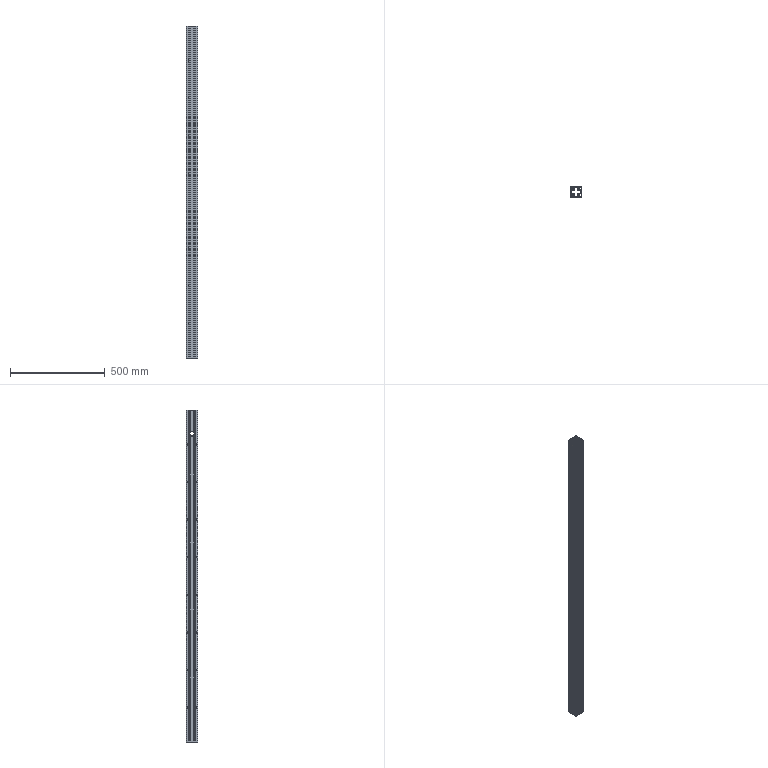Part | STEP file | Industrial aluminium profile 6060 | 1 solid | 2160 faces | box 60 x 60 x 1750 mm | volume 1492239 mm3 | cylinder 1382 | plane 778 | commonest cylinder face diameters 0.6 x694 1.222 x228 6.8 x184 9 x96 15 x64 0.4 x52